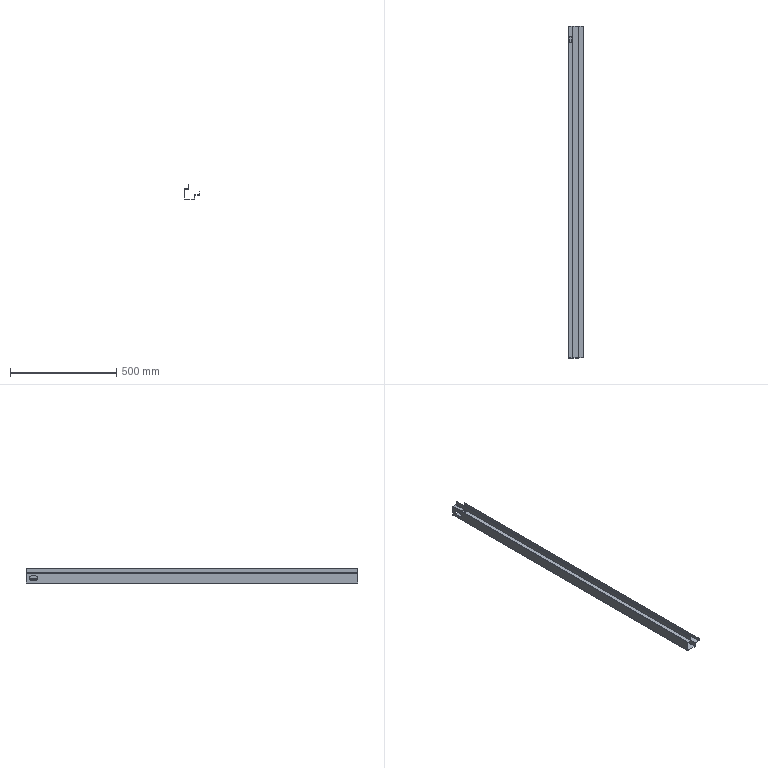Part | SolidWorks | features SplitBody 1 | 1 solid | 66 faces | box 75 x 1562 x 70 mm | volume 454767 mm3 | plane 52 | cylinder 14 | commonest cylinder face diameters 0.2 x6 3.2 x6 20 x2